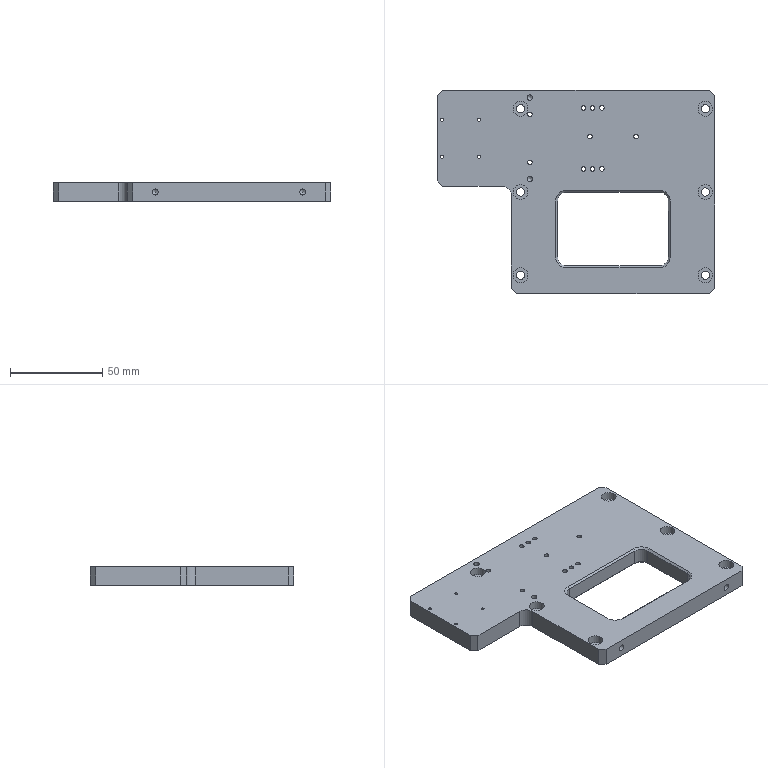CAM job | NX | 3-axis milling, drilling | part box 150 x 110 x 10 mm | stock box 155 x 120 x 12 mm
Tools:
number,name,description,diameter,corner_radius,flute_length,length,flutes
4,D4,平底铣刀-粗,4.0,0.0,25.0,75.0,2
9,D10,平底铣刀-粗,10.0,0.0,35.0,75.0,2
19,D2-J,平底铣刀-精,2.0,0.0,50.0,75.0,2
11,D4-J,平底铣刀-精,4.0,0.0,50.0,75.0,2
7,D6-J,平底铣刀-精,6.0,0.0,25.0,75.0,2
10,D10-J,平底铣刀-精,10.0,0.0,35.0,75.0,2
1,D80R0.8飞刀,圆鼻刀-粗,80.0,0.8,50.0,75.0,2
2,D6倒角刀,倒角刀,6.0,0.0,3.0,25.0,2
18,M2X0.4,丝锥,1.6,0.0,35.0,50.0,2
20,M3X0.5,丝锥,2.5,0.0,35.0,50.0,2
17,ZT1.6,钻头,1.6,0.0,35.0,50.0,2
12,ZT2.5,钻头,2.5,0.0,35.0,50.0,2
17,ZT2.8,钻头,2.8,0.0,35.0,50.0,2
11,ZT4.5,钻头,4.5,0.0,35.0,50.0,2
Operations:
program,operation,operation_type,tool,method,geometry_group,spindle_rpm,surface_speed,feed_per_tooth,feed_cut,feed_plunge,cut_length_mm,path_length_mm,cut_time_min,machine_time_min
B,面铣自动飞面开粗_COPY,FaceMilling,D80R0.8飞刀,分层开粗-切深K-步距G,W-B,4500.0,890.615,0.3333,3000.0,100.0,3202.556,4060.759,1.067,1.153
B,面铣自动飞面精光_COPY,FaceMilling,D80R0.8飞刀,侧刃精光-切深K-步距G,W-B,4500.0,890.615,0.1111,1000.0,100.0,813.0,849.0,0.813,0.8166
B,打点-深0.8,Operation,D6倒角刀,NONE,W-B,8000.0,150.796,0.0312,500.0,90.0,3.6,92.211,0.0072,0.0161
B,盲锥孔-精孔3.0预钻,Operation,ZT2.8,NONE,W-B,3000.0,26.389,0.0133,80.0,90.0,11.603,108.216,0.145,0.1547
B,铣沉头_1,CylinderMilling,D4,METHOD,W-B,8000.0,100.531,0.1125,1800.0,100.0,1086.599,1631.199,0.6037,0.6581
B,铣孔_1,CylinderMilling,D4-J,METHOD,W-B,8000.0,100.531,0.0375,600.0,100.0,105.106,677.906,0.1752,0.2325
B,定点8X45L_COPY,Operation,D6倒角刀,钻孔-切深G-步距G,W-B,4500.0,113.094,0.0556,500.0,100.0,8.4,119.875,0.0168,0.0279
B,钻倒角_3,Operation,D6倒角刀,METHOD,W-B,8000.0,150.796,0.0625,1000.0,0.0,47.5,300.26,0.0475,0.0728
B,钻倒角_4,Operation,D6倒角刀,METHOD,W-B,8000.0,150.796,0.0312,500.0,0.0,9.6,106.302,0.0192,0.0289
B,底壁铣倒角_COPY_COPY,VolumeBased25DMillingOperation,D6倒角刀,爬面_倒角-切深0-步距G,W-B,6500.0,122.519,0.1154,1500.0,100.0,768.939,809.339,0.5126,0.5167
B,平面去毛刺6X45L_COPY,SurfaceContour,D6倒角刀,爬面_倒角-切深0-步距G,W-B,6500.0,122.519,0.1154,1500.0,100.0,669.486,1153.345,0.4463,0.4947
B,铣孔精光D2_1,CylinderMilling,D2-J,精光步距切深关,W-B,8000.0,50.266,0.0125,200.0,100.0,67.653,198.653,0.3383,0.3514
A,顶面,FaceMilling,D80R0.8飞刀,侧刃精光-切深K-步距G,W-A,4000.0,1005.31,0.125,1000.0,100.0,799.0,835.0,0.799,0.8026
A,型腔铣开粗-中_COPY,CavityMilling,D10,分层开粗-切深K-步距G,W-A,8000.0,251.32,0.25,4000.0,100.0,40503.594,41566.237,10.126,10.28
A,框开粗_1,VolumeBased25DMillingOperation,D10,METHOD,W-A,6000.0,188.0,0.25,4000.0,80.0,3026.314,3073.314,0.7566,0.7613
A,打点-深1,Operation,D6倒角刀,NONE,W-A,8000.0,150.796,0.0312,500.0,90.0,36.0,550.028,0.072,0.1234
A,通孔-5-6,Operation,ZT4.5,NONE,W-A,3000.0,42.411,0.025,150.0,90.0,59.712,444.473,0.3981,0.4366
A,通孔-M2螺纹底孔,Operation,ZT1.6,NONE,W-A,3500.0,17.593,0.0043,30.0,90.0,61.923,226.921,2.064,2.081
A,通孔-M3螺纹底孔,Operation,ZT2.5,NONE,W-A,3000.0,23.562,0.05,300.0,90.0,167.511,519.862,0.5584,0.5936
A,框半精_1,VolumeBased25DMillingOperation,D6-J,METHOD,W-A,6000.0,113.0,0.0833,1000.0,100.0,178.607,234.607,0.1786,0.1842
A,框精_1,VolumeBased25DMillingOperation,D6-J,METHOD,W-A,6000.0,113.0,0.0833,1000.0,100.0,178.408,237.408,0.1784,0.1843
A,仅选体,SurfaceContour,D6倒角刀,METHOD,W-A,8000.0,150.796,0.1875,3000.0,100.0,526.366,562.167,0.1755,0.179
A,钻倒角_1,Operation,D6倒角刀,METHOD,W-A,8000.0,150.796,0.0312,500.0,0.0,16.8,143.271,0.0336,0.0462
A,钻倒角_2,Operation,D6倒角刀,METHOD,W-A,8000.0,150.796,0.0312,500.0,0.0,47.5,301.673,0.095,0.1204
A,铣倒角_1,PlanarMilling,D6倒角刀,METHOD,W-A,8000.0,150.796,0.0312,500.0,100.0,104.118,630.124,0.2082,0.2608
A,底壁铣倒角_COPY,VolumeBased25DMillingOperation,D6倒角刀,爬面_倒角-切深0-步距G,W-A,6500.0,122.519,0.1154,1500.0,100.0,768.939,809.339,0.5126,0.5167
A,通孔-攻牙M3,Operation,M3X0.5,METHOD,W-A,800.0,6.283,0.0003,0.5,90.0,140.0,464.84,280.0,280.033
A,通孔-攻牙M2.0,Operation,M2X0.4,METHOD,W-A,1000.0,5.027,0.0002,0.4,90.0,56.0,215.075,140.0,140.016
A,外形半精_2,VolumeBased25DMillingOperation,D10-J,METHOD,W-A,8000.0,251.327,0.0625,1000.0,100.0,545.441,604.441,0.5454,0.5513